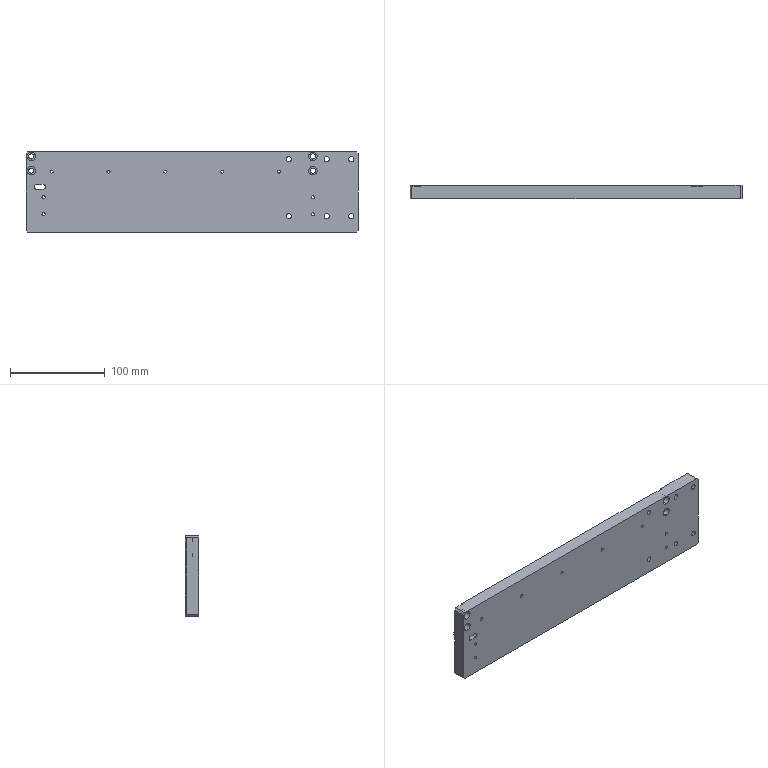Part | STEP file | 1 solid | 100 faces | box 350 x 14 x 85 mm | volume 395442 mm3 | cylinder 64 | plane 36 | commonest cylinder face diameters 5.5 x20 3.3 x18 10 x15 9 x8 5 x2 4 x1